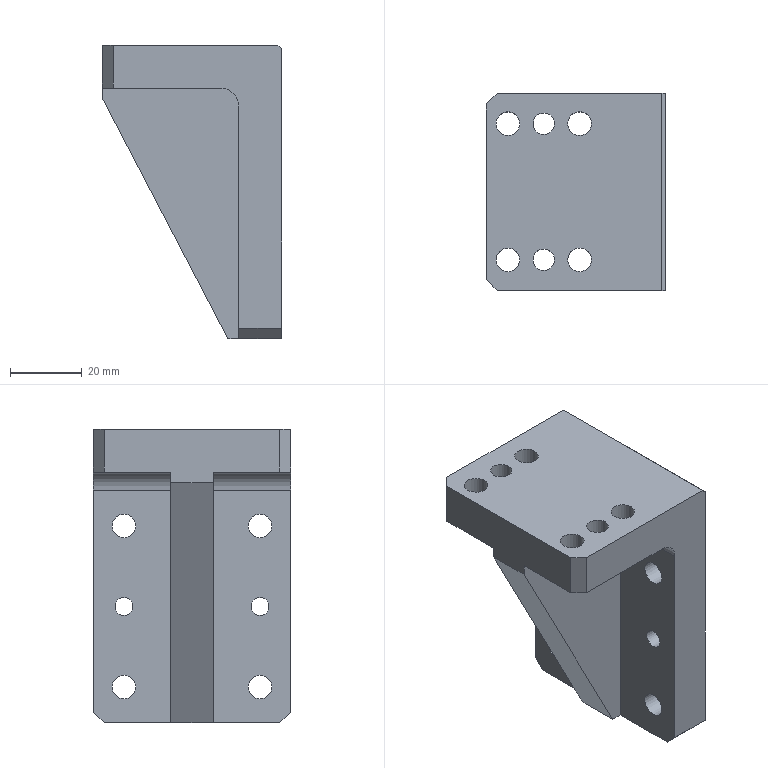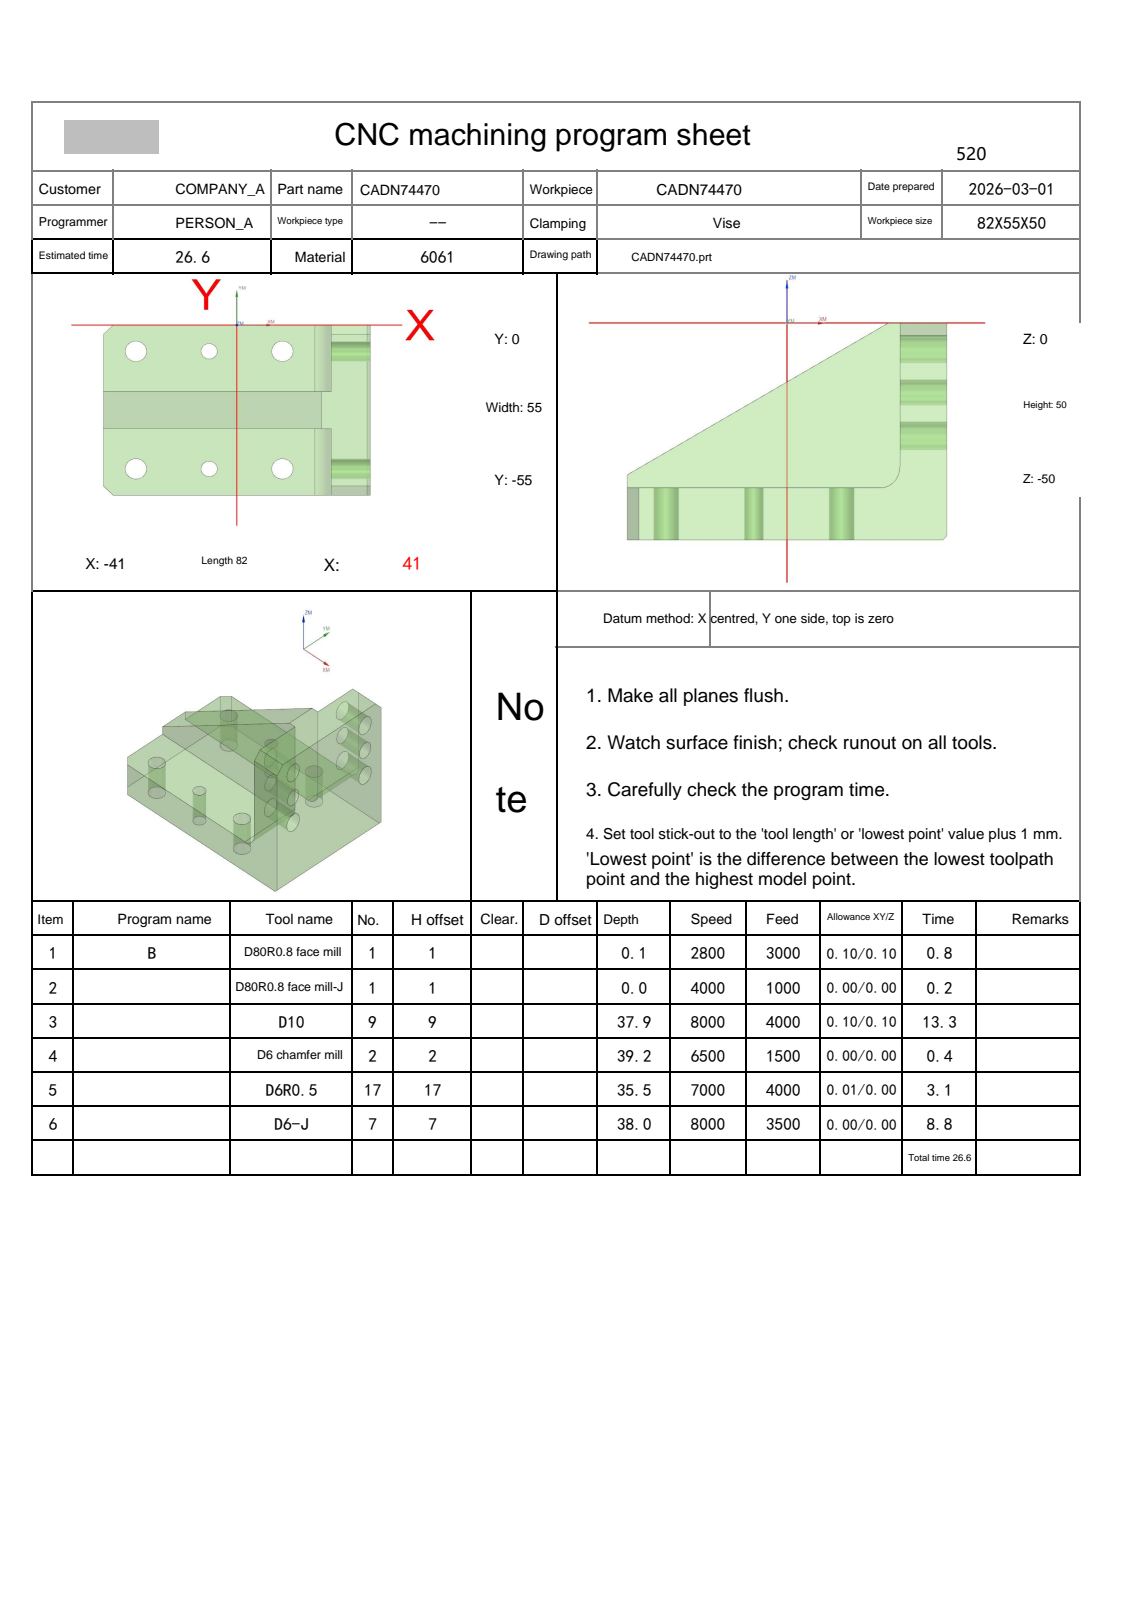NC program | NX | posted by the shop | part box 50 x 55 x 82 mm
Lines 8652 to 10442 of 26562:
N5 T17 M06
(D6R0.5  D=6. R=0.5 H=17 ce=0.01 di=0.00)
G00 G90 G54 X22.709 Y-.34 M03 S7000
G43 H17 Z14.5
M08
Z.429
G01 Z-.071 F4000.
X27.927 Y-.215
X28.052 Y-.212
X42.074
Y-.177 Z-.106
Y-.142 Z-.141
X28.052 Y-.141
X27.926 Y-.144
Y-.106 Z-.177
Y-.074 Z-.212
X28.052 Y-.071
X41.
X42.074
X42.075 Y-.035 Z-.247
Y0.0 Z-.283
X41.
X28.052
X27.925 Y-.003
Y.035 Z-.318
Y.068 Z-.354
X28.052 Y.071
X41.
X42.075
Y.106 Z-.389
Y.141 Z-.424
X41.
X28.052
X27.925 Y.138
X27.924 Y.177 Z-.46
Y.209 Z-.495
X28.052 Y.212
X41.
X42.076
Y.247 Z-.53
Y.283 Z-.566
X41.
X28.052
X27.924 Y.28
Y.318 Z-.601
X27.923 Y.35 Z-.636
X28.052 Y.354
X41.
X42.077 Y.353
Y.389 Z-.672
Y.424 Z-.707
X41.
X28.052
X27.923 Y.421
Y.46 Z-.742
Y.492 Z-.778
X28.052 Y.495
X41.
X42.077
Y.53 Z-.813
X42.078 Y.565 Z-.849
X41. Y.566
X28.052
X27.922 Y.563
Y.601 Z-.884
Y.633 Z-.919
X28.052 Y.636
X41.
X42.078
Y.672 Z-.955
X42.079 Y.707 Z-.99
X41.
X28.052
X27.922 Y.704
X27.921 Y.742 Z-1.025
Y.775 Z-1.061
X28.052 Y.778
X41.
X42.079
Y.813 Z-1.096
Y.848 Z-1.131
X41.
X28.052
X27.921 Y.845
Y.884 Z-1.167
Y.916 Z-1.202
X28.052 Y.919
X41.
X42.079
Y.955 Z-1.237
Y.99 Z-1.273
X41.
X28.052
X27.921 Y.987
Y1.025 Z-1.308
Y1.058 Z-1.344
X28.052 Y1.061
X41.
X42.079 Y1.06
Y1.096 Z-1.379
Y1.131 Z-1.414
X41.
X29.
X27.921
Y1.167 Z-1.45
Y1.199 Z-1.485
X28.052 Y1.202
X41.
X42.079
Y1.237 Z-1.52
Y1.273 Z-1.556
X41.
X28.052
X27.921 Y1.27
Y1.308 Z-1.591
Y1.34 Z-1.626
X28.052 Y1.343
X41.
X42.079
Y1.379 Z-1.662
Y1.414 Z-1.697
X41.
X28.052
X27.921 Y1.411
Y1.45 Z-1.732
Y1.482 Z-1.768
X28.052 Y1.485
X41.
X42.079
Y1.52 Z-1.803
Y1.555 Z-1.838
X41. Y1.556
X28.052
X27.921 Y1.553
Y1.591 Z-1.874
Y1.623 Z-1.909
X28.052 Y1.626
X41.
X42.079
Y1.662 Z-1.945
Y1.697 Z-1.98
X41.
X28.052
X27.921 Y1.694
Y1.732 Z-2.015
Y1.765 Z-2.051
X28.052 Y1.768
X41.
X42.079
Y1.803 Z-2.086
Y1.838 Z-2.121
X41.
X28.052
X27.921 Y1.835
Y1.874 Z-2.157
Y1.906 Z-2.192
X28.052 Y1.909
X41.
X42.079
Y1.944 Z-2.227
Y1.98 Z-2.263
X41.
X28.052
X27.921 Y1.977
X27.922 Y2.015 Z-2.298
Y2.048 Z-2.333
X28.052 Y2.051
X41.
X42.078 Y2.05
Y2.086 Z-2.369
Y2.121 Z-2.404
X41.
X28.052
X27.922 Y2.118
Y2.157 Z-2.44
Y2.189 Z-2.475
X28.052 Y2.192
X41.
X42.077
Y2.227 Z-2.51
Y2.263 Z-2.546
X41.
X28.052
X27.923 Y2.26
Y2.298 Z-2.581
Y2.33 Z-2.616
X28.052 Y2.333
X41.
X42.077
Y2.369 Z-2.652
X42.076 Y2.404 Z-2.687
X41.
X28.052
X27.924 Y2.401
Y2.439 Z-2.722
Y2.472 Z-2.758
X28.052 Y2.475
X41.
X42.076
Y2.51 Z-2.793
Y2.545 Z-2.828
X41. Y2.546
X28.052
X27.924 Y2.543
X27.925 Y2.581 Z-2.864
Y2.613 Z-2.899
X28.052 Y2.616
X41.
X42.075
Y2.652 Z-2.934
Y2.687 Z-2.97
X41.
X28.052
X27.925 Y2.684
Y2.722 Z-3.005
X27.926 Y2.755 Z-3.041
X28.052 Y2.758
X41.
X42.075
X42.074 Y2.793 Z-3.076
Y2.828 Z-3.111
X41.
X28.052
X27.926 Y2.825
Y2.864 Z-3.147
Y2.896 Z-3.182
X42.074 Y2.899
Y2.934 Z-3.217
X42.073 Y2.97 Z-3.253
X27.927 Y2.967
Y3.001 Z-3.284
Y3.029 Z-3.315
X28.052 Y3.032
X42.073 Y3.031
Y3.063 Z-3.345
Y3.093 Z-3.376
X28.052
X27.927 Y3.09
Y3.124 Z-3.407
X27.928 Y3.152 Z-3.438
X42.072 Y3.155
Y3.186 Z-3.469
Y3.217 Z-3.5
X28.052
X27.928 Y3.214
G00 Z14.5
X47.222 Y-54.788
Z.429
G01 Z-.071
X42.074
X28.05
X27.926 Y-54.785
Y-54.823 Z-.106
Y-54.856 Z-.141
X28.05 Y-54.859
X42.074 Y-54.858
Y-54.894 Z-.177
Y-54.929 Z-.212
X41.
X28.05
X27.926 Y-54.926
X27.925 Y-54.965 Z-.247
Y-54.997 Z-.283
X28.05 Y-55.
X41.
X42.075
Y-55.035 Z-.318
Y-55.071 Z-.354
X41.
X28.05
X27.925 Y-55.068
Y-55.106 Z-.389
Y-55.138 Z-.424
X28.05 Y-55.141
X41.
X42.075
X42.076 Y-55.177 Z-.46
Y-55.212 Z-.495
X41.
X28.05
X27.924 Y-55.209
Y-55.247 Z-.53
Y-55.28 Z-.566
X28.05 Y-55.283
X41.
X42.076
Y-55.318 Z-.601
X42.077 Y-55.353 Z-.636
X41. Y-55.354
X28.05
X27.923 Y-55.35
Y-55.389 Z-.672
Y-55.421 Z-.707
X28.05 Y-55.424
X41.
X42.077
Y-55.46 Z-.742
Y-55.495 Z-.778
X41.
X28.05
X27.923 Y-55.492
X27.922 Y-55.53 Z-.813
Y-55.563 Z-.849
X28.05 Y-55.566
X41.
X42.078
Y-55.601 Z-.884
Y-55.636 Z-.919
X41.
X28.05
X27.922 Y-55.633
Y-55.672 Z-.955
Y-55.704 Z-.99
X28.05 Y-55.707
X41.
X42.078
X42.079 Y-55.742 Z-1.025
Y-55.778 Z-1.061
X41.
X28.05
X27.921 Y-55.775
Y-55.813 Z-1.096
Y-55.845 Z-1.131
X28.05 Y-55.848
X41.
X42.079
Y-55.884 Z-1.167
Y-55.919 Z-1.202
X41.
X28.05
X27.921 Y-55.916
Y-55.955 Z-1.237
Y-55.987 Z-1.273
X28.05 Y-55.99
X41.
X42.079
Y-56.025 Z-1.308
Y-56.06 Z-1.344
X41. Y-56.061
X28.05
X27.921 Y-56.058
Y-56.096 Z-1.379
Y-56.131 Z-1.414
X29.
X41.
X42.079
Y-56.167 Z-1.45
Y-56.202 Z-1.485
X41.
X28.05
X27.921 Y-56.199
Y-56.237 Z-1.52
Y-56.27 Z-1.556
X28.05 Y-56.273
X41.
X42.079
Y-56.308 Z-1.591
Y-56.343 Z-1.626
X41.
X28.05
X27.921 Y-56.34
Y-56.379 Z-1.662
Y-56.411 Z-1.697
X28.05 Y-56.414
X41.
X42.079
Y-56.45 Z-1.732
Y-56.485 Z-1.768
X41.
X28.05
X27.921 Y-56.482
Y-56.52 Z-1.803
Y-56.553 Z-1.838
X28.05 Y-56.556
X41.
X42.079 Y-56.555
Y-56.591 Z-1.874
Y-56.626 Z-1.909
X41.
X28.05
X27.921 Y-56.623
Y-56.662 Z-1.945
Y-56.694 Z-1.98
X28.05 Y-56.697
X41.
X42.079
Y-56.732 Z-2.015
Y-56.768 Z-2.051
X41.
X28.05
X27.921 Y-56.765
Y-56.803 Z-2.086
Y-56.835 Z-2.121
X28.05 Y-56.838
X41.
X42.079
Y-56.874 Z-2.157
Y-56.909 Z-2.192
X41.
X28.05
X27.921 Y-56.906
Y-56.944 Z-2.227
Y-56.977 Z-2.263
X28.05 Y-56.98
X41.
X42.079
X42.078 Y-57.015 Z-2.298
Y-57.05 Z-2.333
X41. Y-57.051
X28.05
X27.922 Y-57.048
Y-57.086 Z-2.369
Y-57.118 Z-2.404
X28.05 Y-57.121
X41.
X42.078
Y-57.157 Z-2.44
Y-57.192 Z-2.475
X41.
X28.05
X27.922 Y-57.189
X27.923 Y-57.227 Z-2.51
Y-57.26 Z-2.546
X28.05 Y-57.263
X41.
X42.077
Y-57.298 Z-2.581
Y-57.333 Z-2.616
X41.
X28.05
X27.923 Y-57.33
Y-57.369 Z-2.652
X27.924 Y-57.401 Z-2.687
X28.05 Y-57.404
X41.
X42.076
Y-57.439 Z-2.722
Y-57.475 Z-2.758
X41.
X28.05
X27.924 Y-57.472
Y-57.51 Z-2.793
Y-57.543 Z-2.828
X28.05 Y-57.546
X41.
X42.076 Y-57.545
X42.075 Y-57.581 Z-2.864
Y-57.616 Z-2.899
X41.
X28.05
X27.925 Y-57.613
Y-57.652 Z-2.934
Y-57.684 Z-2.97
X28.05 Y-57.687
X41.
X42.075
Y-57.722 Z-3.005
Y-57.758 Z-3.041
X41.
X28.05
X27.925 Y-57.755
X27.926 Y-57.793 Z-3.076
Y-57.825 Z-3.111
X28.05 Y-57.828
X41.
X42.074
Y-57.864 Z-3.147
Y-57.899 Z-3.182
X28.05
X27.926 Y-57.896
Y-57.934 Z-3.217
X27.927 Y-57.967 Z-3.253
X28.05 Y-57.97
X42.073
Y-58.001 Z-3.284
Y-58.031 Z-3.315
X28.05 Y-58.032
X27.927 Y-58.029
Y-58.063 Z-3.345
Y-58.09 Z-3.376
X28.05 Y-58.093
X42.073
Y-58.124 Z-3.407
Y-58.155 Z-3.438
X28.05
X27.928 Y-58.152
Y-58.186 Z-3.469
Y-58.214 Z-3.5
X28.05 Y-58.217
X42.072
G00 Z14.5
G00 G90 X22.146 Y-38.838 M03 S7000
Z14.5
Z.454
G01 Z-.046 F4000.
X23.329 Y-37.575
X23.281 Y-34.576
X23.279 Y-34.403
Y-20.597
X23.281 Y-20.424
X23.234 Z-.069
X23.193 Z-.093
X23.19 Y-21.5
Y-33.5
X23.193 Y-34.576
X23.146 Z-.116
X23.104 Y-34.577 Z-.139
X23.101 Y-33.5
Y-21.5
X23.104 Y-20.423
X23.057 Z-.162
X23.015 Z-.185
X23.013 Y-21.5
Y-33.5
X23.015 Y-34.577
X22.968 Y-34.578 Z-.208
X22.927 Z-.232
X22.924 Y-33.5
Y-21.5
X22.927 Y-20.422
X22.88 Z-.255
X22.838 Z-.278
X22.835 Y-21.5
Y-33.5
X22.838 Y-34.578
X22.791 Y-34.579 Z-.301
X22.749 Z-.324
X22.747 Y-33.5
Y-21.5
X22.749 Y-20.421
X22.703 Z-.347
X22.661 Y-20.42 Z-.37
X22.658 Y-21.5
Y-33.5
X22.661 Y-34.58
X22.614 Z-.394
X22.572 Z-.417
X22.57 Y-33.5
Y-21.5
X22.572 Y-20.42
X22.525 Z-.44
X22.484 Y-20.419 Z-.463
X22.481 Y-21.5
Y-33.5
X22.484 Y-34.581
X22.437 Z-.486
X22.395 Z-.509
X22.392 Y-33.5
Y-21.5
X22.395 Y-20.419
X22.348 Y-20.418 Z-.532
X22.306 Z-.556
X22.304 Y-21.5
Y-33.5
X22.306 Y-34.582
X22.259 Z-.579
X22.218 Z-.602
X22.215 Y-33.5
Y-21.5
X22.218 Y-20.418
X22.171 Y-20.417 Z-.625
X22.129 Z-.648
X22.126 Y-21.5
Y-33.5
X22.129 Y-34.583
X22.082 Z-.671
X22.04 Y-34.584 Z-.695
X22.038 Y-33.5
Y-21.5
X22.04 Y-20.417
X21.993 Y-20.416 Z-.718
X21.952 Z-.741
X21.949 Y-21.5
Y-33.5
X21.952 Y-34.584
X21.905 Z-.764
X21.863 Y-34.585 Z-.787
X21.86 Y-33.5
Y-21.5
X21.863 Y-20.415
X21.816 Z-.81
X21.774 Z-.833
X21.772 Y-21.5
Y-33.5
X21.774 Y-34.585
X21.728 Y-34.586 Z-.857
X21.686 Z-.88
X21.683 Y-33.5
Y-21.5
X21.686 Y-20.414
X21.639 Z-.903
X21.597 Z-.926
X21.595 Y-21.5
Y-33.5
X21.597 Y-34.586
X21.55 Y-34.587 Z-.949
X21.508 Z-.972
X21.506 Y-33.5
Y-21.5
X21.508 Y-20.413
X21.462 Z-.995
X21.42 Z-1.019
X21.417 Y-21.5
Y-33.5
X21.42 Y-34.587
X21.373 Z-1.042
X21.331 Y-34.588 Z-1.065
X21.329 Y-33.5
Y-21.5
X21.331 Y-20.412
X21.284 Z-1.088
X21.243 Z-1.111
X21.24 Y-21.5
Y-33.5
X21.243 Y-34.588
X21.196 Z-1.134
X21.154 Y-34.589 Z-1.158
X21.151 Y-33.5
Y-21.5
X21.154 Y-20.411
X21.107 Z-1.181
X21.065 Z-1.204
X21.063 Y-21.5
Y-33.5
X21.065 Y-34.589
X21.018 Z-1.227
X20.977 Z-1.25
X20.974 Y-33.5
Y-21.5
X20.977 Y-20.411
X20.93 Z-1.273
X20.888 Y-20.41 Z-1.296
X20.885 Y-21.5
Y-33.5
X20.888 Y-34.59
X20.841 Z-1.32
X20.799 Z-1.343
X20.797 Y-33.5
Y-21.5
X20.799 Y-20.41
X20.753 Z-1.366
X20.711 Y-20.409 Z-1.389
X20.708 Y-21.5
Y-33.5
X20.711 Y-34.59
X20.664 Y-34.591 Z-1.412
X20.622 Z-1.435
X20.62 Y-33.5
Y-21.5
X20.622 Y-20.409
X20.575 Z-1.459
X20.533 Z-1.482
X20.531 Y-21.5
Y-33.5
X20.533 Y-34.591
X20.487 Z-1.505
X20.445 Y-34.592 Z-1.528
X20.442 Y-33.5
Y-21.5
X20.445 Y-20.408
X20.398 Z-1.551
X20.356 Z-1.574
X20.354 Y-21.5
Y-33.5
X20.356 Y-34.592
X20.309 Z-1.597
X20.267 Z-1.621
X20.265 Y-33.5
Y-21.5
X20.267 Y-20.408
X20.221 Y-20.407 Z-1.644
X20.179 Z-1.667
X20.176 Y-21.5
Y-33.5
X20.179 Y-34.593
X20.132 Z-1.69
X20.09 Z-1.713
X20.088 Y-33.5
Y-21.5
X20.09 Y-20.407
X20.043 Z-1.736
X20.002 Y-20.406 Z-1.759
X19.999 Y-21.5
Y-33.5
X20.002 Y-34.593
X19.955 Y-34.594 Z-1.783
X19.913 Z-1.806
X19.911 Y-33.5
Y-21.5
X19.913 Y-20.406
X19.866 Z-1.829
X19.824 Z-1.852
X19.822 Y-21.5
Y-33.5
X19.824 Y-34.594
X19.778 Z-1.875
X19.736 Y-34.595 Z-1.898
X19.733 Y-33.5
Y-21.5
X19.736 Y-20.405
X19.689 Z-1.922
X19.647 Z-1.945
X19.645 Y-21.5
Y-33.5
X19.647 Y-34.595
X19.6 Z-1.968
X19.558 Z-1.991
X19.556 Y-33.5
Y-21.5
X19.558 Y-20.405
X19.512 Z-2.014
X19.47 Z-2.037
X19.467 Y-21.5
Y-33.5
X19.47 Y-34.595
X19.423 Z-2.06
X19.381 Z-2.084
X19.379 Y-33.5
Y-21.5
X19.381 Y-20.405
X19.334 Z-2.107
X19.292 Y-20.404 Z-2.13
X19.29 Y-21.5
Y-33.5
X19.292 Y-34.596
X19.246 Z-2.153
X19.204 Z-2.176
X19.201 Y-33.5
Y-21.5
X19.204 Y-20.404
X19.157 Z-2.199
X19.115 Z-2.222
X19.113 Y-21.5
Y-33.5
X19.115 Y-34.596
X19.068 Z-2.246
X19.027 Z-2.269
X19.024 Y-33.5
Y-21.5
X19.027 Y-20.404
X18.98 Z-2.292
X18.938 Z-2.315
X18.936 Y-21.5
Y-33.5
X18.938 Y-34.596
X18.891 Z-2.338
X18.849 Y-34.597 Z-2.361
X18.847 Y-33.5
Y-21.5
X18.849 Y-20.404
X18.803 Y-20.403 Z-2.385
X18.761 Z-2.408
X18.758 Y-21.5
Y-33.5
X18.761 Y-34.597
X18.714 Z-2.431
X18.672 Z-2.454
X18.67 Y-33.5
Y-21.5
X18.672 Y-20.403
X18.625 Z-2.477
X18.583 Z-2.5
X18.581 Y-21.5
Y-33.5
X18.583 Y-34.597
X18.537 Z-2.523
X18.495 Z-2.547
X18.492 Y-33.5
Y-21.5
X18.495 Y-20.403
X18.448 Z-2.57
X18.406 Y-20.402 Z-2.593
X18.404 Y-21.5
Y-33.5
X18.406 Y-34.597
X18.359 Z-2.616
X18.317 Y-34.598 Z-2.639
X18.315 Y-33.5
Y-21.5
X18.317 Y-20.402
X18.271 Z-2.662
X18.229 Z-2.686
X18.226 Y-21.5
Y-33.5
X18.229 Y-34.598
X18.182 Z-2.709
X18.14 Z-2.732
X18.138 Y-33.5
Y-21.5
X18.14 Y-20.402
X18.093 Z-2.755
X18.052 Z-2.778
X18.049 Y-21.5
Y-33.5
X18.052 Y-34.598
X18.005 Z-2.801
X17.963 Z-2.824
X17.961 Y-33.5
Y-21.5
X17.963 Y-20.402
X17.916 Z-2.848
X17.874 Z-2.871
X17.872 Y-21.5
Y-33.5
X17.874 Y-34.598
X17.828 Z-2.894
X17.786 Z-2.917
X17.783 Y-33.5
Y-21.5
X17.786 Y-20.402
X17.739 Z-2.94
X17.697 Z-2.963
X17.695 Y-21.5
Y-33.5
X17.697 Y-34.599
X17.65 Z-2.986
X17.608 Z-3.01
X17.606 Y-33.5
Y-21.5
X17.608 Y-20.401
X17.562 Z-3.033
X17.52 Z-3.056
X17.517 Y-21.5
Y-33.5
X17.52 Y-34.599
X17.473 Z-3.079
X17.431 Z-3.102
X17.429 Y-33.5
Y-21.5
X17.431 Y-20.401
X17.384 Z-3.125
X17.342 Z-3.149
X17.34 Y-21.5
Y-33.5
X17.342 Y-34.599
X17.296 Z-3.172
X17.254 Z-3.195
X17.251 Y-33.5
Y-21.5
X17.254 Y-20.401
X17.207 Z-3.218
X17.165 Z-3.241
X17.163 Y-21.5
Y-33.5
X17.165 Y-34.599
X17.119 Z-3.264
X17.077 Z-3.287
X17.074 Y-33.5
Y-21.5
X17.077 Y-20.401
X17.03 Z-3.311
X16.988 Z-3.334
X16.986 Y-21.5
Y-33.5
X16.988 Y-34.599
X16.941 Z-3.357
X16.899 Z-3.38
X16.897 Y-33.5
Y-21.5
X16.899 Y-20.401
X16.853 Z-3.403
X16.811 Z-3.426
X16.808 Y-21.5
Y-33.5
X16.811 Y-34.599
X16.764 Z-3.449
X16.722 Z-3.473
X16.72 Y-33.5
Y-21.5
X16.722 Y-20.401
X16.675 Z-3.496
X16.633 Z-3.519
X16.631 Y-21.5
Y-33.5
X16.633 Y-34.599
X16.587 Z-3.542
X16.545 Z-3.565
X16.542 Y-33.5
Y-21.5
X16.545 Y-20.401
X16.498 Z-3.588
X16.456 Z-3.612
X16.454 Y-21.5
Y-33.5
X16.456 Y-34.599
X16.409 Z-3.635
X16.367 Z-3.658
X16.365 Y-33.5
Y-21.5
X16.367 Y-20.401
X16.321 Z-3.681
X16.279 Z-3.704
X16.276 Y-21.5
Y-33.5
X16.279 Y-34.599
X16.232 Z-3.727
X16.19 Z-3.75
X16.188 Y-33.5
Y-21.5
X16.19 Y-20.4
X16.144 Z-3.774
X16.102 Z-3.797
X16.099 Y-21.5
Y-33.5
X16.102 Y-34.599
X16.055 Z-3.82
X16.013 Z-3.843
X16.011 Y-33.5
Y-21.5
X16.013 Y-20.4
X15.966 Z-3.866
X15.924 Z-3.889
X15.922 Y-21.5
Y-33.5
X15.924 Y-34.599
X15.878 Z-3.913
X15.836 Z-3.936
X15.833 Y-33.5
Y-21.5
X15.836 Y-20.4
X15.789 Z-3.959
X15.747 Z-3.982
X15.745 Y-21.5
Y-33.5
X15.747 Y-34.599
X15.7 Z-4.005
X15.658 Y-34.6 Z-4.028
X15.656 Y-33.5
Y-21.5
X15.658 Y-20.4
X15.612 Z-4.051
X15.57 Z-4.075
X15.567 Y-21.5
Y-33.5
X15.57 Y-34.6
X15.523 Z-4.098
X15.481 Z-4.121
X15.479 Y-33.5
Y-21.5
X15.481 Y-20.4
X15.434 Z-4.144
X15.392 Z-4.167
X15.39 Y-21.5
Y-33.5
X15.392 Y-34.6
X15.346 Z-4.19
X15.304 Z-4.213
X15.301 Y-33.5
Y-21.5
X15.304 Y-20.4
X15.257 Z-4.237
X15.215 Z-4.26
X15.213 Y-21.5
Y-33.5
X15.215 Y-34.6
X15.169 Z-4.283
X15.127 Z-4.306
X15.124 Y-33.5
Y-21.5
X15.127 Y-20.4
X15.08 Z-4.329
X15.038 Z-4.352
X15.036 Y-21.5
Y-33.5
X15.038 Y-34.6
X14.991 Z-4.376
X14.949 Z-4.399
X14.947 Y-33.5
Y-21.5
X14.949 Y-20.4
X14.903 Z-4.422
X14.861 Z-4.445
X14.858 Y-21.5
Y-33.5
X14.861 Y-34.6
X14.814 Z-4.468
X14.772 Z-4.491
X14.77 Y-33.5
Y-21.5
X14.772 Y-20.4
X14.725 Z-4.514
X14.683 Z-4.538
X14.681 Y-21.5
Y-33.5
X14.683 Y-34.6
X14.637 Z-4.561
X14.595 Z-4.584
X14.592 Y-33.5
Y-21.5
X14.595 Y-20.4
X14.548 Z-4.607
X14.506 Z-4.63
X14.504 Y-21.5
Y-33.5
X14.506 Y-34.6
X14.459 Z-4.653
X14.417 Z-4.676
X14.415 Y-33.5
Y-21.5
X14.417 Y-20.4
X14.371 Z-4.7
X14.329 Z-4.723
X14.327 Y-21.5
Y-33.5
X14.329 Y-34.6
X14.282 Z-4.746
X14.24 Z-4.769
X14.238 Y-33.5
Y-21.5
X14.24 Y-20.4
X14.194 Z-4.792
X14.152 Z-4.815
X14.149 Y-21.5
Y-33.5
X14.152 Y-34.6
X14.105 Z-4.839
X14.061 Z-4.862
Y-33.5
Y-21.5
Y-20.4
X14.016 Z-4.885
X13.974 Z-4.908
X13.972 Y-21.5
Y-33.5
X13.974 Y-34.6
X13.928 Z-4.931
X13.886 Z-4.954
X13.883 Y-33.5
Y-21.5
X13.886 Y-20.4
X13.839 Z-4.977
X13.797 Z-5.001
X13.795 Y-21.5
Y-33.5
X13.797 Y-34.6
X13.75 Z-5.024
X13.708 Z-5.047
X13.706 Y-33.5
Y-21.5
X13.708 Y-20.4
X13.662 Z-5.07
X13.62 Z-5.093
X13.617 Y-21.5
Y-33.5
X13.62 Y-34.6
X13.573 Z-5.116
X13.531 Z-5.14
X13.529 Y-33.5
Y-21.5
X13.531 Y-20.4
X13.484 Z-5.163
X13.442 Z-5.186
X13.44 Y-21.5
Y-33.5
X13.442 Y-34.6
X13.396 Z-5.209
X13.354 Z-5.232
X13.352 Y-33.5
Y-21.5
X13.354 Y-20.4
X13.307 Z-5.255
X13.265 Z-5.278
X13.263 Y-21.5
Y-33.5
X13.265 Y-34.6
X13.219 Z-5.302
X13.177 Z-5.325
X13.174 Y-33.5
Y-21.5
X13.177 Y-20.4
X13.13 Z-5.348
X13.088 Z-5.371
X13.086 Y-21.5
Y-33.5
X13.088 Y-34.6
X13.041 Z-5.394
X12.999 Z-5.417
X12.997 Y-33.5
Y-21.5
X12.999 Y-20.4
X12.953 Z-5.44
X12.911 Z-5.464
X12.908 Y-21.5
Y-33.5
X12.911 Y-34.6
X12.864 Z-5.487
X12.822 Z-5.51
X12.82 Y-33.5
Y-21.5
X12.822 Y-20.4
X12.775 Z-5.533
X12.733 Z-5.556
X12.731 Y-21.5
Y-33.5
X12.733 Y-34.6
X12.687 Z-5.579
X12.645 Z-5.603
X12.642 Y-33.5
Y-21.5
X12.645 Y-20.4
X12.598 Z-5.626
X12.556 Z-5.649
X12.554 Y-21.5
Y-33.5
X12.556 Y-34.6
X12.509 Z-5.672
X12.467 Z-5.695
X12.465 Y-33.5
Y-21.5
X12.467 Y-20.4
X12.421 Z-5.718
X12.379 Z-5.741
X12.377 Y-21.5
Y-33.5
X12.379 Y-34.6
X12.332 Z-5.765
X12.29 Z-5.788
X12.288 Y-33.5
Y-21.5
X12.29 Y-20.4
X12.244 Z-5.811
X12.202 Z-5.834
X12.199 Y-21.5
Y-33.5
X12.202 Y-34.6
X12.155 Z-5.857
X12.113 Z-5.88
X12.111 Y-33.5
Y-21.5
X12.113 Y-20.4
X12.066 Z-5.903
X12.024 Z-5.927
X12.022 Y-21.5
Y-33.5
X12.024 Y-34.6
X11.978 Z-5.95
X11.936 Z-5.973
X11.933 Y-33.5
Y-21.5
X11.936 Y-20.4
X11.889 Z-5.996
X11.847 Z-6.019
X11.845 Y-21.5
Y-33.5
X11.847 Y-34.6
X11.8 Z-6.042
X11.758 Z-6.066
X11.756 Y-33.5
Y-21.5
X11.758 Y-20.4
X11.712 Z-6.089
X11.67 Z-6.112
X11.667 Y-21.5
Y-33.5
X11.67 Y-34.6
X11.623 Z-6.135
X11.581 Z-6.158
X11.579 Y-33.5
Y-21.5
X11.581 Y-20.4
X11.535 Z-6.181
X11.492 Z-6.204
X11.49 Y-21.5
Y-33.5
X11.492 Y-34.6
X11.446 Z-6.228
X11.404 Z-6.251
X11.402 Y-33.5
Y-21.5
X11.404 Y-20.4
X11.357 Z-6.274
X11.315 Z-6.297
X11.313 Y-21.5
Y-33.5
X11.315 Y-34.6
X11.269 Z-6.32
X11.227 Z-6.343
X11.224 Y-33.5
Y-21.5
X11.227 Y-20.4
X11.18 Z-6.366
X11.138 Z-6.39
X11.136 Y-21.5
Y-33.5
X11.138 Y-34.6
X11.091 Z-6.413
X11.049 Z-6.436
X11.047 Y-33.5
Y-21.5
X11.049 Y-20.4
X11.003 Z-6.459
X10.961 Z-6.482
X10.958 Y-21.5
Y-33.5
X10.961 Y-34.6
X10.914 Z-6.505
X10.872 Z-6.529
X10.87 Y-33.5
Y-21.5
X10.872 Y-20.4
X10.825 Z-6.552
X10.783 Z-6.575
X10.781 Y-21.5
Y-33.5
X10.783 Y-34.6
X10.737 Z-6.598
X10.695 Z-6.621
X10.692 Y-33.5
Y-21.5
X10.695 Y-20.4
X10.648 Z-6.644
X10.606 Z-6.667
X10.604 Y-21.5
Y-33.5
X10.606 Y-34.6
X10.56 Z-6.691
X10.518 Z-6.714
X10.515 Y-33.5
Y-21.5
X10.518 Y-20.4
X10.471 Z-6.737
X10.429 Z-6.76
X10.427 Y-21.5
Y-33.5
X10.429 Y-34.6
X10.382 Z-6.783
X10.34 Z-6.806
X10.338 Y-33.5
Y-21.5
X10.34 Y-20.4
X10.294 Z-6.83
X10.25 Z-6.853
X10.249 Y-21.5
Y-33.5
X10.25 Y-34.6
X10.205 Z-6.876
X10.163 Z-6.899
X10.161 Y-33.5
Y-21.5
X10.163 Y-20.4
X10.116 Z-6.922
X10.074 Z-6.945
X10.072 Y-21.5
Y-33.5
X10.074 Y-34.6
X10.028 Z-6.968
X9.986 Z-6.992
X9.983 Y-33.5
Y-21.5
X9.986 Y-20.4
X9.939 Z-7.015
X9.897 Z-7.038
X9.895 Y-21.5
Y-33.5
X9.897 Y-34.6
X9.85 Z-7.061
X9.808 Z-7.084
X9.806 Y-33.5
Y-21.5
X9.808 Y-20.4
X9.762 Z-7.107
X9.72 Z-7.13
X9.717 Y-21.5
Y-33.5
X9.72 Y-34.6
X9.673 Z-7.154
X9.631 Z-7.177
X9.629 Y-33.5
Y-21.5
X9.631 Y-20.4
X9.585 Z-7.2
X9.543 Z-7.223
X9.54 Y-21.5
Y-33.5
X9.543 Y-34.6
X9.496 Z-7.246
X9.454 Z-7.269
X9.452 Y-33.5
Y-21.5
X9.454 Y-20.4
X9.407 Z-7.293
X9.365 Z-7.316
X9.363 Y-21.5
Y-33.5
X9.365 Y-34.6
X9.319 Z-7.339
X9.277 Z-7.362
X9.274 Y-33.5
Y-21.5
X9.277 Y-20.4
X9.23 Z-7.385
X9.188 Z-7.408
X9.186 Y-21.5
Y-33.5
X9.188 Y-34.6
X9.141 Z-7.431
X9.099 Z-7.455
X9.097 Y-33.5
Y-21.5
X9.099 Y-20.4
X9.053 Z-7.478
X9.011 Z-7.501
X9.008 Y-21.5
Y-33.5
X9.011 Y-34.6
X8.964 Z-7.524
X8.922 Z-7.547
X8.92 Y-33.5
Y-21.5
X8.922 Y-20.4
X8.875 Z-7.57
X8.833 Z-7.593
X8.831 Y-21.5
Y-33.5
X8.833 Y-34.6
X8.787 Z-7.617
X8.745 Z-7.64
X8.743 Y-33.5
Y-21.5
X8.745 Y-20.4
X8.698 Z-7.663
X8.656 Z-7.686
X8.654 Y-21.5
Y-33.5
X8.656 Y-34.6
X8.61 Z-7.709
X8.568 Z-7.732
X8.565 Y-33.5
Y-21.5
X8.568 Y-20.4
X8.521 Z-7.756
X8.479 Z-7.779
X8.477 Y-21.5
Y-33.5
X8.479 Y-34.6
X8.432 Z-7.802
X8.39 Z-7.825
X8.388 Y-33.5
Y-21.5
X8.39 Y-20.4
X8.344 Z-7.848
X8.302 Z-7.871
X8.299 Y-21.5
Y-33.5
X8.302 Y-34.6
X8.255 Z-7.894
X8.213 Z-7.918
X8.211 Y-33.5
Y-21.5
X8.213 Y-20.4
X8.166 Z-7.941
X8.124 Z-7.964
X8.122 Y-21.5
Y-33.5
X8.124 Y-34.6
X8.078 Z-7.987
X8.036 Z-8.01
X8.033 Y-33.5
Y-21.5
X8.036 Y-20.4
X7.989 Z-8.033
X7.947 Z-8.057
X7.945 Y-21.5
Y-33.5
X7.947 Y-34.6
X7.9 Z-8.08
X7.858 Z-8.103
X7.856 Y-33.5
Y-21.5
X7.858 Y-20.4
X7.812 Z-8.126
X7.77 Z-8.149
X7.768 Y-21.5
Y-33.5
X7.77 Y-34.6
X7.723 Z-8.172
X7.681 Z-8.195
X7.679 Y-33.5
Y-21.5
X7.681 Y-20.4
X7.635 Z-8.219
X7.593 Z-8.242
X7.59 Y-21.5
Y-33.5
X7.593 Y-34.6
X7.546 Z-8.265
X7.504 Z-8.288
X7.502 Y-33.5
Y-21.5
X7.504 Y-20.4
X7.457 Z-8.311
X7.415 Z-8.334
X7.413 Y-21.5
Y-33.5
X7.415 Y-34.6
X7.369 Z-8.357
X7.327 Z-8.381
X7.324 Y-33.5
Y-21.5
X7.327 Y-20.4
X7.28 Z-8.404
X7.238 Z-8.427
X7.236 Y-21.5
Y-33.5
X7.238 Y-34.6
X7.191 Z-8.45
X7.149 Z-8.473
X7.147 Y-33.5
Y-21.5
X7.149 Y-20.4
X7.103 Z-8.496
X7.061 Z-8.52
X7.058 Y-21.5
Y-33.5
X7.061 Y-34.6
X7.014 Z-8.543
X6.972 Z-8.566
X6.97 Y-33.5
Y-21.5
X6.972 Y-20.4
X6.926 Z-8.589
X6.883 Z-8.612
X6.881 Y-21.5
Y-33.5
X6.883 Y-34.6
X6.837 Z-8.635
X6.795 Z-8.658
X6.793 Y-33.5
Y-21.5
X6.795 Y-20.4
X6.748 Z-8.682
X6.706 Z-8.705
X6.704 Y-21.5
Y-33.5
X6.706 Y-34.6
X6.66 Z-8.728
X6.618 Z-8.751
X6.615 Y-33.5
Y-21.5
X6.618 Y-20.4
X6.571 Z-8.774
X6.529 Z-8.797
X6.527 Y-21.5
Y-33.5
X6.529 Y-34.6
X6.482 Z-8.82
X6.439 Z-8.844
X6.438 Y-33.5
Y-21.5
X6.439 Y-20.4
X6.394 Z-8.867
X6.352 Z-8.89
X6.349 Y-21.5
Y-33.5
X6.352 Y-34.6
X6.305 Z-8.913
X6.263 Z-8.936
X6.261 Y-33.5
Y-21.5
X6.263 Y-20.4
X6.216 Z-8.959
X6.174 Z-8.983
X6.172 Y-21.5
Y-33.5
X6.174 Y-34.6
X6.128 Z-9.006
X6.086 Z-9.029
X6.083 Y-33.5
Y-21.5
X6.086 Y-20.4
X6.039 Z-9.052
X5.997 Z-9.075
X5.995 Y-21.5
Y-33.5
X5.997 Y-34.6
X5.951 Z-9.098
X5.908 Z-9.121
X5.906 Y-33.5
Y-21.5
X5.908 Y-20.4
X5.862 Z-9.145
X5.82 Z-9.168
X5.818 Y-21.5
Y-33.5
X5.82 Y-34.6
X5.773 Z-9.191
X5.731 Z-9.214
X5.729 Y-33.5
Y-21.5
X5.731 Y-20.4
X5.685 Z-9.237
X5.643 Z-9.26
X5.64 Y-21.5
Y-33.5
X5.643 Y-34.6
X5.596 Z-9.284
X5.554 Z-9.307
X5.552 Y-33.5
Y-21.5
X5.554 Y-20.4
X5.507 Z-9.33
X5.465 Z-9.353
X5.463 Y-21.5
Y-33.5
X5.465 Y-34.6
X5.419 Z-9.376
X5.377 Z-9.399
X5.374 Y-33.5
Y-21.5
X5.377 Y-20.4
X5.33 Z-9.422
X5.288 Z-9.446
X5.286 Y-21.5
Y-33.5
X5.288 Y-34.6
X5.241 Z-9.469
X5.199 Z-9.492
X5.197 Y-33.5
Y-21.5
X5.199 Y-20.4
X5.153 Z-9.515
X5.111 Z-9.538
X5.108 Y-21.5
Y-33.5
X5.111 Y-34.6
X5.064 Z-9.561
X5.022 Z-9.584
X5.02 Y-33.5
Y-21.5
X5.022 Y-20.4
X4.976 Z-9.608
X4.934 Z-9.631
X4.931 Y-21.5
Y-33.5
X4.934 Y-34.6
X4.887 Z-9.654
X4.845 Z-9.677
X4.843 Y-33.5
Y-21.5
X4.845 Y-20.4
X4.798 Z-9.7
X4.756 Z-9.723
X4.754 Y-21.5
Y-33.5
X4.756 Y-34.6
X4.71 Z-9.747
X4.668 Z-9.77
X4.665 Y-33.5
Y-21.5
X4.668 Y-20.4
X4.621 Z-9.793
X4.579 Z-9.816
X4.577 Y-21.5
Y-33.5
X4.579 Y-34.6
X4.532 Z-9.839
X4.49 Z-9.862
X4.488 Y-33.5
Y-21.5
X4.49 Y-20.4
X4.444 Z-9.885
X4.402 Z-9.909
X4.399 Y-21.5
Y-33.5
X4.402 Y-34.6
X4.355 Z-9.932
X4.313 Z-9.955
X4.311 Y-33.5
Y-21.5
X4.313 Y-20.4
X4.266 Z-9.978
X4.224 Z-10.001
X4.222 Y-21.5
Y-33.5
X4.224 Y-34.6
X4.178 Z-10.024
X4.136 Z-10.047
X4.134 Y-33.5
Y-21.5
X4.136 Y-20.4
X4.089 Z-10.071
X4.047 Z-10.094
X4.045 Y-21.5
Y-33.5
X4.047 Y-34.6
X4.001 Z-10.117
X3.959 Z-10.14
X3.956 Y-33.5
Y-21.5
X3.959 Y-20.4
X3.912 Z-10.163
X3.87 Z-10.186
X3.868 Y-21.5
Y-33.5
X3.87 Y-34.6
X3.823 Z-10.21
X3.781 Z-10.233
X3.779 Y-33.5
Y-21.5
X3.781 Y-20.4
X3.735 Z-10.256
X3.693 Z-10.279
X3.69 Y-21.5
Y-33.5
X3.693 Y-34.6
X3.646 Z-10.302
X3.604 Z-10.325
X3.602 Y-33.5
Y-21.5
X3.604 Y-20.4
X3.557 Z-10.348
X3.515 Z-10.372
X3.513 Y-21.5
Y-33.5
X3.515 Y-34.6
X3.469 Z-10.395
X3.427 Z-10.418
X3.424 Y-33.5
Y-21.5
X3.427 Y-20.4
X3.38 Z-10.441
X3.338 Z-10.464
X3.336 Y-21.5
Y-33.5
X3.338 Y-34.6
X3.291 Z-10.487
X3.249 Z-10.511
X3.247 Y-33.5
Y-21.5
X3.249 Y-20.4
X3.203 Z-10.534
X3.161 Z-10.557
X3.159 Y-21.5
Y-33.5
X3.161 Y-34.6
X3.114 Z-10.58
X3.072 Z-10.603
X3.07 Y-33.5
Y-21.5
X3.072 Y-20.4
X3.026 Z-10.626
X2.984 Z-10.649
X2.981 Y-21.5
Y-33.5
X2.984 Y-34.6
X2.937 Z-10.673
X2.895 Z-10.696
X2.893 Y-33.5
Y-21.5
X2.895 Y-20.4
X2.848 Z-10.719
X2.806 Z-10.742
X2.804 Y-21.5
Y-33.5
X2.806 Y-34.6
X2.76 Z-10.765
X2.718 Z-10.788
X2.715 Y-33.5
Y-21.5
X2.718 Y-20.4
X2.671 Z-10.811
X2.629 Z-10.835
X2.627 Y-21.5
Y-33.5
X2.629 Y-34.6
X2.582 Z-10.858
X2.54 Z-10.881
X2.538 Y-33.5
Y-21.5
X2.54 Y-20.4
X2.494 Z-10.904
X2.452 Z-10.927
X2.449 Y-21.5
Y-33.5
X2.452 Y-34.6
X2.405 Z-10.95
X2.363 Z-10.974
X2.361 Y-33.5
Y-21.5
X2.363 Y-20.4
X2.316 Z-10.997
X2.274 Z-11.02
X2.272 Y-21.5
Y-33.5
X2.274 Y-34.6
X2.228 Z-11.043
X2.186 Z-11.066
X2.184 Y-33.5
Y-21.5
X2.186 Y-20.4
X2.139 Z-11.089
X2.097 Z-11.112
X2.095 Y-21.5
Y-33.5
X2.097 Y-34.6
X2.051 Z-11.136
X2.009 Z-11.159
X2.006 Y-33.5
Y-21.5
X2.009 Y-20.4
X1.962 Z-11.182
X1.92 Z-11.205
X1.918 Y-21.5
Y-33.5
X1.92 Y-34.6
X1.873 Z-11.228
X1.831 Z-11.251
X1.829 Y-33.5
Y-21.5
X1.831 Y-20.4
X1.785 Z-11.274
X1.743 Z-11.298
X1.74 Y-21.5
Y-33.5
X1.743 Y-34.6
X1.696 Z-11.321
X1.654 Z-11.344
X1.652 Y-33.5
Y-21.5
X1.654 Y-20.4
X1.607 Z-11.367
X1.565 Z-11.39
X1.563 Y-21.5
Y-33.5
X1.565 Y-34.6
X1.519 Z-11.413
X1.477 Z-11.437
X1.474 Y-33.5
Y-21.5
X1.477 Y-20.4
X1.43 Z-11.46
X1.388 Z-11.483
X1.386 Y-21.5
Y-33.5
X1.388 Y-34.6
X1.342 Z-11.506
X1.299 Z-11.529
X1.297 Y-33.5
Y-21.5
X1.299 Y-20.4
X1.253 Z-11.552
X1.211 Z-11.575
X1.209 Y-21.5
Y-33.5
X1.211 Y-34.6
X1.164 Z-11.599
X1.122 Z-11.622
X1.12 Y-33.5
Y-21.5
X1.122 Y-20.4
X1.076 Z-11.645
X1.034 Z-11.668
X1.031 Y-21.5
Y-33.5
X1.034 Y-34.6
X.987 Z-11.691
X.945 Z-11.714
X.943 Y-33.5
Y-21.5
X.945 Y-20.4
X.898 Z-11.738
X.856 Z-11.761
X.854 Y-21.5
Y-33.5
X.856 Y-34.6
X.81 Z-11.784
X.768 Z-11.807
X.765 Y-33.5
Y-21.5
X.768 Y-20.4
X.721 Z-11.83
X.679 Z-11.853
X.677 Y-21.5
Y-33.5
X.679 Y-34.6
X.632 Z-11.876
X.59 Z-11.9
X.588 Y-33.5
Y-21.5
X.59 Y-20.4
X.544 Z-11.923
X.502 Z-11.946
X.499 Y-21.5
Y-33.5
X.502 Y-34.6
X.455 Z-11.969
X.413 Z-11.992
X.411 Y-33.5
Y-21.5
X.413 Y-20.4
X.367 Z-12.015